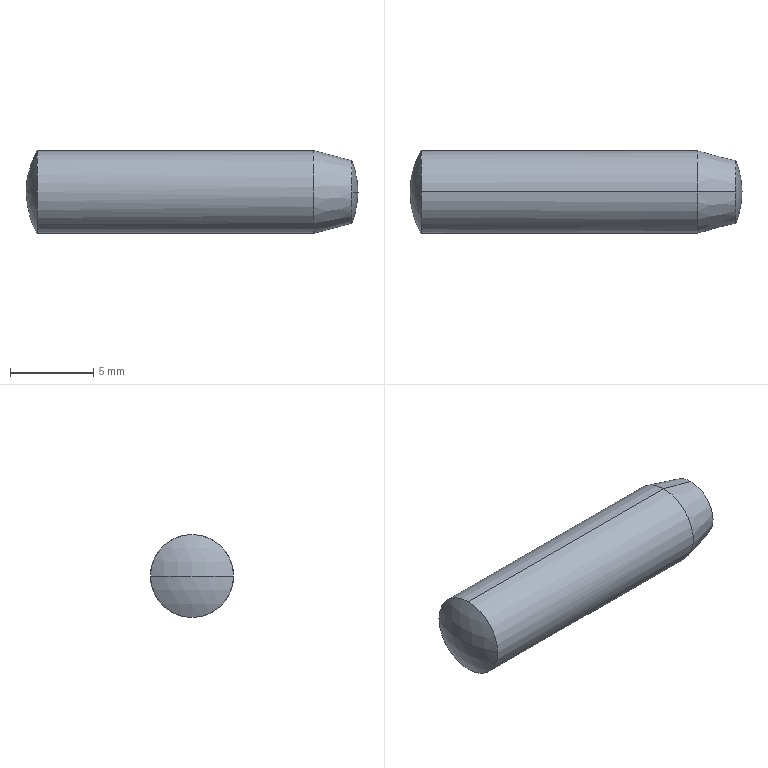Part | NX | features BREP 1 | 1 solid | 8 faces | box 20 x 5 x 5 mm | volume 370.896 mm3 | sphere 4 | cone 2 | cylinder 2 | commonest cylinder face diameters 5 x2
STEP:
#1=CARTESIAN_POINT('',(9.632,-1.883,0.));
#2=VERTEX_POINT('',#1);
#3=CARTESIAN_POINT('',(10.,0.,0.));
#4=VERTEX_POINT('',#3);
#5=CARTESIAN_POINT('',(5.,0.,0.));
#6=DIRECTION('',(0.,0.,-1.));
#7=DIRECTION('',(-1.,0.,0.));
#8=AXIS2_PLACEMENT_3D('',#5,#6,#7);
#9=CIRCLE('',#8,5.);
#10=EDGE_CURVE('',#2,#4,#9,.F.);
#11=ORIENTED_EDGE('',*,*,#10,.T.);
#12=CARTESIAN_POINT('',(9.632,1.883,0.));
#13=VERTEX_POINT('',#12);
#14=CARTESIAN_POINT('',(5.,0.,0.));
#15=DIRECTION('',(0.,0.,1.));
#16=DIRECTION('',(0.,-1.,0.));
#17=AXIS2_PLACEMENT_3D('',#14,#15,#16);
#18=CIRCLE('',#17,5.);
#19=EDGE_CURVE('',#13,#4,#18,.F.);
#20=ORIENTED_EDGE('',*,*,#19,.F.);
#21=CARTESIAN_POINT('',(9.632,0.,1.883));
#22=VERTEX_POINT('',#21);
#23=CARTESIAN_POINT('',(9.632,0.,0.));
#24=DIRECTION('',(-1.,0.,0.));
#25=DIRECTION('',(0.,0.,1.));
#26=AXIS2_PLACEMENT_3D('',#23,#24,#25);
#27=CIRCLE('',#26,1.883);
#28=EDGE_CURVE('',#22,#13,#27,.T.);
#29=ORIENTED_EDGE('',*,*,#28,.F.);
#30=CARTESIAN_POINT('',(9.632,0.,0.));
#31=DIRECTION('',(-1.,0.,0.));
#32=DIRECTION('',(0.,0.,1.));
#33=AXIS2_PLACEMENT_3D('',#30,#31,#32);
#34=CIRCLE('',#33,1.883);
#35=EDGE_CURVE('',#2,#22,#34,.T.);
#36=ORIENTED_EDGE('',*,*,#35,.F.);
#37=EDGE_LOOP('',(#11,#20,#29,#36));
#38=FACE_BOUND('',#37,.T.);
#39=CARTESIAN_POINT('',(5.,0.,0.));
#40=DIRECTION('',(0.,0.,1.));
#41=DIRECTION('',(0.,1.,0.));
#42=AXIS2_PLACEMENT_3D('',#39,#40,#41);
#43=SPHERICAL_SURFACE('',#42,5.);
#44=ADVANCED_FACE('',(#38),#43,.T.);
#45=ORIENTED_EDGE('',*,*,#28,.T.);
#46=CARTESIAN_POINT('',(9.632,0.,-1.883));
#47=VERTEX_POINT('',#46);
#48=CARTESIAN_POINT('',(9.632,0.,0.));
#49=DIRECTION('',(-1.,0.,0.));
#50=DIRECTION('',(0.,0.,1.));
#51=AXIS2_PLACEMENT_3D('',#48,#49,#50);
#52=CIRCLE('',#51,1.883);
#53=EDGE_CURVE('',#13,#47,#52,.T.);
#54=ORIENTED_EDGE('',*,*,#53,.T.);
#55=CARTESIAN_POINT('',(7.33,0.,-2.5));
#56=VERTEX_POINT('',#55);
#57=CARTESIAN_POINT('',(9.632,0.,-1.883));
#58=DIRECTION('',(-0.9659,0.,-0.2588));
#59=VECTOR('',#58,1000.);
#60=LINE('',#57,#59);
#61=EDGE_CURVE('',#47,#56,#60,.T.);
#62=ORIENTED_EDGE('',*,*,#61,.T.);
#63=CARTESIAN_POINT('',(7.33,0.,2.5));
#64=VERTEX_POINT('',#63);
#65=CARTESIAN_POINT('',(7.33,0.,0.));
#66=DIRECTION('',(-1.,0.,0.));
#67=DIRECTION('',(0.,0.,1.));
#68=AXIS2_PLACEMENT_3D('',#65,#66,#67);
#69=CIRCLE('',#68,2.5);
#70=EDGE_CURVE('',#64,#56,#69,.T.);
#71=ORIENTED_EDGE('',*,*,#70,.F.);
#72=CARTESIAN_POINT('',(9.632,0.,1.883));
#73=DIRECTION('',(-0.9659,0.,0.2588));
#74=VECTOR('',#73,1000.);
#75=LINE('',#72,#74);
#76=EDGE_CURVE('',#22,#64,#75,.T.);
#77=ORIENTED_EDGE('',*,*,#76,.F.);
#78=EDGE_LOOP('',(#45,#54,#62,#71,#77));
#79=FACE_BOUND('',#78,.T.);
#80=CARTESIAN_POINT('',(9.632,0.,0.));
#81=DIRECTION('',(-1.,0.,0.));
#82=DIRECTION('',(0.,0.,-1.));
#83=AXIS2_PLACEMENT_3D('',#80,#81,#82);
#84=CONICAL_SURFACE('',#83,1.883,0.2618);
#85=ADVANCED_FACE('',(#79),#84,.T.);
#86=ORIENTED_EDGE('',*,*,#70,.T.);
#87=CARTESIAN_POINT('',(-9.33,0.,-2.5));
#88=VERTEX_POINT('',#87);
#89=CARTESIAN_POINT('',(10.,0.,-2.5));
#90=DIRECTION('',(-1.,0.,0.));
#91=VECTOR('',#90,1000.);
#92=LINE('',#89,#91);
#93=EDGE_CURVE('',#56,#88,#92,.T.);
#94=ORIENTED_EDGE('',*,*,#93,.T.);
#95=CARTESIAN_POINT('',(-9.33,2.5,0.));
#96=VERTEX_POINT('',#95);
#97=CARTESIAN_POINT('',(-9.33,0.,0.));
#98=DIRECTION('',(-1.,0.,0.));
#99=DIRECTION('',(0.,0.,1.));
#100=AXIS2_PLACEMENT_3D('',#97,#98,#99);
#101=CIRCLE('',#100,2.5);
#102=EDGE_CURVE('',#96,#88,#101,.T.);
#103=ORIENTED_EDGE('',*,*,#102,.F.);
#104=CARTESIAN_POINT('',(-9.33,0.,2.5));
#105=VERTEX_POINT('',#104);
#106=CARTESIAN_POINT('',(-9.33,0.,0.));
#107=DIRECTION('',(-1.,0.,0.));
#108=DIRECTION('',(0.,0.,1.));
#109=AXIS2_PLACEMENT_3D('',#106,#107,#108);
#110=CIRCLE('',#109,2.5);
#111=EDGE_CURVE('',#105,#96,#110,.T.);
#112=ORIENTED_EDGE('',*,*,#111,.F.);
#113=CARTESIAN_POINT('',(10.,0.,2.5));
#114=DIRECTION('',(-1.,0.,0.));
#115=VECTOR('',#114,1000.);
#116=LINE('',#113,#115);
#117=EDGE_CURVE('',#64,#105,#116,.T.);
#118=ORIENTED_EDGE('',*,*,#117,.F.);
#119=EDGE_LOOP('',(#86,#94,#103,#112,#118));
#120=FACE_BOUND('',#119,.T.);
#121=CARTESIAN_POINT('',(10.,0.,0.));
#122=DIRECTION('',(-1.,0.,0.));
#123=DIRECTION('',(0.,0.,-1.));
#124=AXIS2_PLACEMENT_3D('',#121,#122,#123);
#125=CYLINDRICAL_SURFACE('',#124,2.5);
#126=ADVANCED_FACE('',(#120),#125,.T.);
#127=ORIENTED_EDGE('',*,*,#102,.T.);
#128=CARTESIAN_POINT('',(-9.33,-2.5,0.));
#129=VERTEX_POINT('',#128);
#130=CARTESIAN_POINT('',(-9.33,0.,0.));
#131=DIRECTION('',(-1.,0.,0.));
#132=DIRECTION('',(0.,0.,1.));
#133=AXIS2_PLACEMENT_3D('',#130,#131,#132);
#134=CIRCLE('',#133,2.5);
#135=EDGE_CURVE('',#88,#129,#134,.T.);
#136=ORIENTED_EDGE('',*,*,#135,.T.);
#137=CARTESIAN_POINT('',(-10.,0.,0.));
#138=VERTEX_POINT('',#137);
#139=CARTESIAN_POINT('',(-5.,0.,0.));
#140=DIRECTION('',(0.,0.,-1.));
#141=DIRECTION('',(0.,1.,0.));
#142=AXIS2_PLACEMENT_3D('',#139,#140,#141);
#143=CIRCLE('',#142,5.);
#144=EDGE_CURVE('',#129,#138,#143,.T.);
#145=ORIENTED_EDGE('',*,*,#144,.T.);
#146=CARTESIAN_POINT('',(-5.,0.,0.));
#147=DIRECTION('',(0.,0.,1.));
#148=DIRECTION('',(1.,0.,0.));
#149=AXIS2_PLACEMENT_3D('',#146,#147,#148);
#150=CIRCLE('',#149,5.);
#151=EDGE_CURVE('',#96,#138,#150,.T.);
#152=ORIENTED_EDGE('',*,*,#151,.F.);
#153=EDGE_LOOP('',(#127,#136,#145,#152));
#154=FACE_BOUND('',#153,.T.);
#155=CARTESIAN_POINT('',(-5.,0.,0.));
#156=DIRECTION('',(0.,0.,-1.));
#157=DIRECTION('',(0.,-1.,0.));
#158=AXIS2_PLACEMENT_3D('',#155,#156,#157);
#159=SPHERICAL_SURFACE('',#158,5.);
#160=ADVANCED_FACE('',(#154),#159,.T.);
#161=ORIENTED_EDGE('',*,*,#144,.F.);
#162=CARTESIAN_POINT('',(-9.33,0.,0.));
#163=DIRECTION('',(-1.,0.,0.));
#164=DIRECTION('',(0.,0.,1.));
#165=AXIS2_PLACEMENT_3D('',#162,#163,#164);
#166=CIRCLE('',#165,2.5);
#167=EDGE_CURVE('',#129,#105,#166,.T.);
#168=ORIENTED_EDGE('',*,*,#167,.T.);
#169=ORIENTED_EDGE('',*,*,#111,.T.);
#170=ORIENTED_EDGE('',*,*,#151,.T.);
#171=EDGE_LOOP('',(#161,#168,#169,#170));
#172=FACE_BOUND('',#171,.T.);
#173=CARTESIAN_POINT('',(-5.,0.,0.));
#174=DIRECTION('',(0.,0.,-1.));
#175=DIRECTION('',(0.,-1.,0.));
#176=AXIS2_PLACEMENT_3D('',#173,#174,#175);
#177=SPHERICAL_SURFACE('',#176,5.);
#178=ADVANCED_FACE('',(#172),#177,.T.);
#179=ORIENTED_EDGE('',*,*,#93,.F.);
#180=CARTESIAN_POINT('',(7.33,0.,0.));
#181=DIRECTION('',(-1.,0.,0.));
#182=DIRECTION('',(0.,0.,1.));
#183=AXIS2_PLACEMENT_3D('',#180,#181,#182);
#184=CIRCLE('',#183,2.5);
#185=EDGE_CURVE('',#56,#64,#184,.T.);
#186=ORIENTED_EDGE('',*,*,#185,.T.);
#187=ORIENTED_EDGE('',*,*,#117,.T.);
#188=ORIENTED_EDGE('',*,*,#167,.F.);
#189=ORIENTED_EDGE('',*,*,#135,.F.);
#190=EDGE_LOOP('',(#179,#186,#187,#188,#189));
#191=FACE_BOUND('',#190,.T.);
#192=CARTESIAN_POINT('',(10.,0.,0.));
#193=DIRECTION('',(-1.,0.,0.));
#194=DIRECTION('',(0.,0.,-1.));
#195=AXIS2_PLACEMENT_3D('',#192,#193,#194);
#196=CYLINDRICAL_SURFACE('',#195,2.5);
#197=ADVANCED_FACE('',(#191),#196,.T.);
#198=ORIENTED_EDGE('',*,*,#61,.F.);
#199=CARTESIAN_POINT('',(9.632,0.,0.));
#200=DIRECTION('',(-1.,0.,0.));
#201=DIRECTION('',(0.,0.,1.));
#202=AXIS2_PLACEMENT_3D('',#199,#200,#201);
#203=CIRCLE('',#202,1.883);
#204=EDGE_CURVE('',#47,#2,#203,.T.);
#205=ORIENTED_EDGE('',*,*,#204,.T.);
#206=ORIENTED_EDGE('',*,*,#35,.T.);
#207=ORIENTED_EDGE('',*,*,#76,.T.);
#208=ORIENTED_EDGE('',*,*,#185,.F.);
#209=EDGE_LOOP('',(#198,#205,#206,#207,#208));
#210=FACE_BOUND('',#209,.T.);
#211=CARTESIAN_POINT('',(9.632,0.,0.));
#212=DIRECTION('',(-1.,0.,0.));
#213=DIRECTION('',(0.,0.,-1.));
#214=AXIS2_PLACEMENT_3D('',#211,#212,#213);
#215=CONICAL_SURFACE('',#214,1.883,0.2618);
#216=ADVANCED_FACE('',(#210),#215,.T.);
#217=ORIENTED_EDGE('',*,*,#19,.T.);
#218=ORIENTED_EDGE('',*,*,#10,.F.);
#219=ORIENTED_EDGE('',*,*,#204,.F.);
#220=ORIENTED_EDGE('',*,*,#53,.F.);
#221=EDGE_LOOP('',(#217,#218,#219,#220));
#222=FACE_BOUND('',#221,.T.);
#223=CARTESIAN_POINT('',(5.,0.,0.));
#224=DIRECTION('',(0.,0.,1.));
#225=DIRECTION('',(0.,1.,0.));
#226=AXIS2_PLACEMENT_3D('',#223,#224,#225);
#227=SPHERICAL_SURFACE('',#226,5.);
#228=ADVANCED_FACE('',(#222),#227,.T.);
#229=CLOSED_SHELL('',(#44,#85,#126,#160,#178,#197,#216,#228));
#230=MANIFOLD_SOLID_BREP('',#229);
#231=(LENGTH_UNIT()NAMED_UNIT(*)SI_UNIT(.MILLI.,.METRE.));
#232=UNCERTAINTY_MEASURE_WITH_UNIT(LENGTH_MEASURE(0.00001),#231,'','');
#233=(NAMED_UNIT(*)PLANE_ANGLE_UNIT()SI_UNIT($,.RADIAN.));
#234=(NAMED_UNIT(*)SI_UNIT($,.STERADIAN.)SOLID_ANGLE_UNIT());
#235=(GEOMETRIC_REPRESENTATION_CONTEXT(3)GLOBAL_UNCERTAINTY_ASSIGNED_CONTEXT((#232))GLOBAL_UNIT_ASSIGNED_CONTEXT((#231,#233,#234))REPRESENTATION_CONTEXT('',''));
#236=ADVANCED_BREP_SHAPE_REPRESENTATION('',(#230),#235);